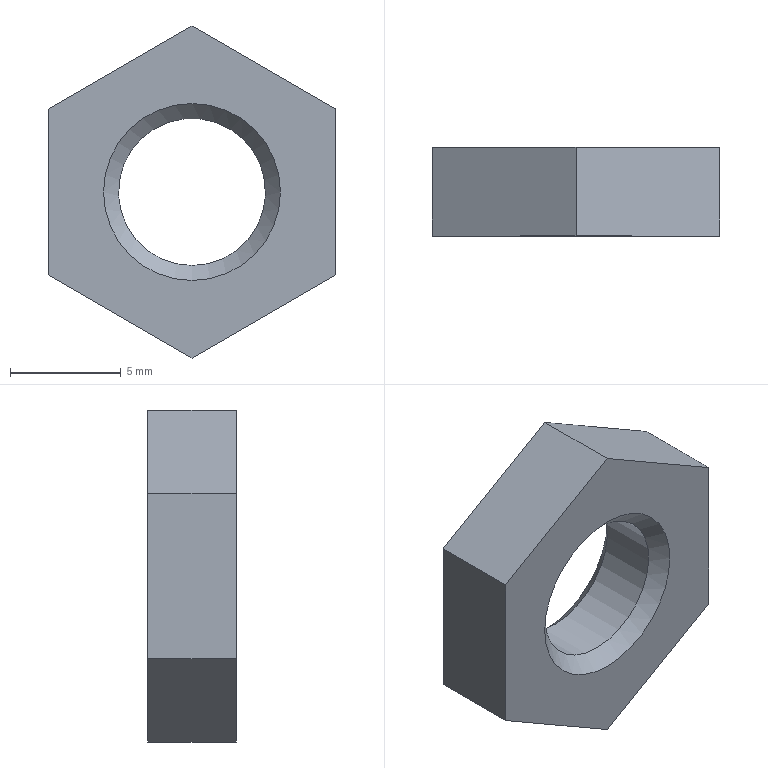Part | STEP file | 1 solid | 11 faces | box 13 x 4 x 15.011 mm | volume 436.424 mm3 | plane 8 | cone 2 | cylinder 1 | commonest cylinder face diameters 6.647 x1
STEP:
#1=CARTESIAN_POINT('',(0.,0.,0.));
#2=DIRECTION('',(0.,0.,1.));
#3=DIRECTION('',(1.,0.,0.));
#4=AXIS2_PLACEMENT_3D('',#1,#2,#3);
#5=CARTESIAN_POINT('',(0.,0.,7.506));
#6=VERTEX_POINT('',#5);
#7=CARTESIAN_POINT('',(6.5,0.,3.753));
#8=VERTEX_POINT('',#7);
#9=CARTESIAN_POINT('',(0.,0.,7.506));
#10=DIRECTION('',(0.866,0.,-0.5));
#11=VECTOR('',#10,1.);
#12=LINE('',#9,#11);
#13=CARTESIAN_POINT('',(0.,0.,7.506));
#14=DIRECTION('',(0.5,0.,0.866));
#15=DIRECTION('',(0.866,0.,-0.5));
#16=AXIS2_PLACEMENT_3D('',#13,#14,#15);
#17=PLANE('',#16);
#18=CARTESIAN_POINT('',(0.,0.));
#19=DIRECTION('',(1.,0.));
#20=VECTOR('',#19,1.);
#21=LINE('',#18,#20);
#22=(GEOMETRIC_REPRESENTATION_CONTEXT(2)PARAMETRIC_REPRESENTATION_CONTEXT()REPRESENTATION_CONTEXT('',''));
#23=DEFINITIONAL_REPRESENTATION('',(#21),#22);
#24=PCURVE('',#17,#23);
#25=CARTESIAN_POINT('',(0.,0.,0.));
#26=DIRECTION('',(0.,1.,0.));
#27=DIRECTION('',(0.,0.,1.));
#28=AXIS2_PLACEMENT_3D('',#25,#26,#27);
#29=PLANE('',#28);
#30=CARTESIAN_POINT('',(7.506,0.));
#31=DIRECTION('',(-0.5,0.866));
#32=VECTOR('',#31,1.);
#33=LINE('',#30,#32);
#34=(GEOMETRIC_REPRESENTATION_CONTEXT(2)PARAMETRIC_REPRESENTATION_CONTEXT()REPRESENTATION_CONTEXT('',''));
#35=DEFINITIONAL_REPRESENTATION('',(#33),#34);
#36=PCURVE('',#29,#35);
#37=SURFACE_CURVE('',#12,(#24,#36),.PCURVE_S1.);
#38=EDGE_CURVE('',#6,#8,#37,.T.);
#39=ORIENTED_EDGE('',*,*,#38,.F.);
#40=CARTESIAN_POINT('',(0.,-4.,7.506));
#41=VERTEX_POINT('',#40);
#42=CARTESIAN_POINT('',(0.,0.,7.506));
#43=DIRECTION('',(0.,-1.,0.));
#44=VECTOR('',#43,1.);
#45=LINE('',#42,#44);
#46=CARTESIAN_POINT('',(0.,0.));
#47=DIRECTION('',(0.,-1.));
#48=VECTOR('',#47,1.);
#49=LINE('',#46,#48);
#50=(GEOMETRIC_REPRESENTATION_CONTEXT(2)PARAMETRIC_REPRESENTATION_CONTEXT()REPRESENTATION_CONTEXT('',''));
#51=DEFINITIONAL_REPRESENTATION('',(#49),#50);
#52=PCURVE('',#17,#51);
#53=CARTESIAN_POINT('',(-6.5,0.,3.753));
#54=DIRECTION('',(-0.5,0.,0.866));
#55=DIRECTION('',(0.866,0.,0.5));
#56=AXIS2_PLACEMENT_3D('',#53,#54,#55);
#57=PLANE('',#56);
#58=CARTESIAN_POINT('',(7.506,0.));
#59=DIRECTION('',(0.,-1.));
#60=VECTOR('',#59,1.);
#61=LINE('',#58,#60);
#62=(GEOMETRIC_REPRESENTATION_CONTEXT(2)PARAMETRIC_REPRESENTATION_CONTEXT()REPRESENTATION_CONTEXT('',''));
#63=DEFINITIONAL_REPRESENTATION('',(#61),#62);
#64=PCURVE('',#57,#63);
#65=SURFACE_CURVE('',#45,(#52,#64),.PCURVE_S1.);
#66=EDGE_CURVE('',#6,#41,#65,.T.);
#67=ORIENTED_EDGE('',*,*,#66,.T.);
#68=CARTESIAN_POINT('',(6.5,-4.,3.753));
#69=VERTEX_POINT('',#68);
#70=CARTESIAN_POINT('',(0.,-4.,7.506));
#71=DIRECTION('',(0.866,0.,-0.5));
#72=VECTOR('',#71,1.);
#73=LINE('',#70,#72);
#74=CARTESIAN_POINT('',(0.,-4.));
#75=DIRECTION('',(1.,0.));
#76=VECTOR('',#75,1.);
#77=LINE('',#74,#76);
#78=(GEOMETRIC_REPRESENTATION_CONTEXT(2)PARAMETRIC_REPRESENTATION_CONTEXT()REPRESENTATION_CONTEXT('',''));
#79=DEFINITIONAL_REPRESENTATION('',(#77),#78);
#80=PCURVE('',#17,#79);
#81=CARTESIAN_POINT('',(0.,-4.,0.));
#82=DIRECTION('',(0.,1.,0.));
#83=DIRECTION('',(0.,0.,1.));
#84=AXIS2_PLACEMENT_3D('',#81,#82,#83);
#85=PLANE('',#84);
#86=CARTESIAN_POINT('',(7.506,0.));
#87=DIRECTION('',(-0.5,0.866));
#88=VECTOR('',#87,1.);
#89=LINE('',#86,#88);
#90=(GEOMETRIC_REPRESENTATION_CONTEXT(2)PARAMETRIC_REPRESENTATION_CONTEXT()REPRESENTATION_CONTEXT('',''));
#91=DEFINITIONAL_REPRESENTATION('',(#89),#90);
#92=PCURVE('',#85,#91);
#93=SURFACE_CURVE('',#73,(#80,#92),.PCURVE_S1.);
#94=EDGE_CURVE('',#41,#69,#93,.T.);
#95=ORIENTED_EDGE('',*,*,#94,.T.);
#96=CARTESIAN_POINT('',(6.5,0.,3.753));
#97=DIRECTION('',(0.,-1.,0.));
#98=VECTOR('',#97,1.);
#99=LINE('',#96,#98);
#100=CARTESIAN_POINT('',(7.506,0.));
#101=DIRECTION('',(0.,-1.));
#102=VECTOR('',#101,1.);
#103=LINE('',#100,#102);
#104=(GEOMETRIC_REPRESENTATION_CONTEXT(2)PARAMETRIC_REPRESENTATION_CONTEXT()REPRESENTATION_CONTEXT('',''));
#105=DEFINITIONAL_REPRESENTATION('',(#103),#104);
#106=PCURVE('',#17,#105);
#107=CARTESIAN_POINT('',(6.5,0.,3.753));
#108=DIRECTION('',(1.,0.,0.));
#109=DIRECTION('',(0.,0.,-1.));
#110=AXIS2_PLACEMENT_3D('',#107,#108,#109);
#111=PLANE('',#110);
#112=CARTESIAN_POINT('',(0.,0.));
#113=DIRECTION('',(0.,-1.));
#114=VECTOR('',#113,1.);
#115=LINE('',#112,#114);
#116=(GEOMETRIC_REPRESENTATION_CONTEXT(2)PARAMETRIC_REPRESENTATION_CONTEXT()REPRESENTATION_CONTEXT('',''));
#117=DEFINITIONAL_REPRESENTATION('',(#115),#116);
#118=PCURVE('',#111,#117);
#119=SURFACE_CURVE('',#99,(#106,#118),.PCURVE_S1.);
#120=EDGE_CURVE('',#8,#69,#119,.T.);
#121=ORIENTED_EDGE('',*,*,#120,.F.);
#122=EDGE_LOOP('',(#39,#67,#95,#121));
#123=FACE_BOUND('',#122,.T.);
#124=ADVANCED_FACE('',(#123),#17,.T.);
#125=CARTESIAN_POINT('',(-6.5,0.,-3.753));
#126=VERTEX_POINT('',#125);
#127=CARTESIAN_POINT('',(-6.5,0.,3.753));
#128=VERTEX_POINT('',#127);
#129=CARTESIAN_POINT('',(-6.5,0.,-3.753));
#130=DIRECTION('',(0.,0.,1.));
#131=VECTOR('',#130,1.);
#132=LINE('',#129,#131);
#133=CARTESIAN_POINT('',(-3.753,-6.5));
#134=DIRECTION('',(1.,0.));
#135=VECTOR('',#134,1.);
#136=LINE('',#133,#135);
#137=(GEOMETRIC_REPRESENTATION_CONTEXT(2)PARAMETRIC_REPRESENTATION_CONTEXT()REPRESENTATION_CONTEXT('',''));
#138=DEFINITIONAL_REPRESENTATION('',(#136),#137);
#139=PCURVE('',#29,#138);
#140=CARTESIAN_POINT('',(-6.5,0.,-3.753));
#141=DIRECTION('',(-1.,0.,0.));
#142=DIRECTION('',(0.,0.,1.));
#143=AXIS2_PLACEMENT_3D('',#140,#141,#142);
#144=PLANE('',#143);
#145=CARTESIAN_POINT('',(0.,0.));
#146=DIRECTION('',(1.,0.));
#147=VECTOR('',#146,1.);
#148=LINE('',#145,#147);
#149=(GEOMETRIC_REPRESENTATION_CONTEXT(2)PARAMETRIC_REPRESENTATION_CONTEXT()REPRESENTATION_CONTEXT('',''));
#150=DEFINITIONAL_REPRESENTATION('',(#148),#149);
#151=PCURVE('',#144,#150);
#152=SURFACE_CURVE('',#132,(#139,#151),.PCURVE_S1.);
#153=EDGE_CURVE('',#126,#128,#152,.T.);
#154=ORIENTED_EDGE('',*,*,#153,.T.);
#155=CARTESIAN_POINT('',(-6.5,0.,3.753));
#156=DIRECTION('',(0.866,0.,0.5));
#157=VECTOR('',#156,1.);
#158=LINE('',#155,#157);
#159=CARTESIAN_POINT('',(3.753,-6.5));
#160=DIRECTION('',(0.5,0.866));
#161=VECTOR('',#160,1.);
#162=LINE('',#159,#161);
#163=(GEOMETRIC_REPRESENTATION_CONTEXT(2)PARAMETRIC_REPRESENTATION_CONTEXT()REPRESENTATION_CONTEXT('',''));
#164=DEFINITIONAL_REPRESENTATION('',(#162),#163);
#165=PCURVE('',#29,#164);
#166=CARTESIAN_POINT('',(0.,0.));
#167=DIRECTION('',(1.,0.));
#168=VECTOR('',#167,1.);
#169=LINE('',#166,#168);
#170=(GEOMETRIC_REPRESENTATION_CONTEXT(2)PARAMETRIC_REPRESENTATION_CONTEXT()REPRESENTATION_CONTEXT('',''));
#171=DEFINITIONAL_REPRESENTATION('',(#169),#170);
#172=PCURVE('',#57,#171);
#173=SURFACE_CURVE('',#158,(#165,#172),.PCURVE_S1.);
#174=EDGE_CURVE('',#128,#6,#173,.T.);
#175=ORIENTED_EDGE('',*,*,#174,.T.);
#176=ORIENTED_EDGE('',*,*,#38,.T.);
#177=CARTESIAN_POINT('',(6.5,0.,-3.753));
#178=VERTEX_POINT('',#177);
#179=CARTESIAN_POINT('',(6.5,0.,3.753));
#180=DIRECTION('',(0.,0.,-1.));
#181=VECTOR('',#180,1.);
#182=LINE('',#179,#181);
#183=CARTESIAN_POINT('',(3.753,6.5));
#184=DIRECTION('',(-1.,0.));
#185=VECTOR('',#184,1.);
#186=LINE('',#183,#185);
#187=(GEOMETRIC_REPRESENTATION_CONTEXT(2)PARAMETRIC_REPRESENTATION_CONTEXT()REPRESENTATION_CONTEXT('',''));
#188=DEFINITIONAL_REPRESENTATION('',(#186),#187);
#189=PCURVE('',#29,#188);
#190=CARTESIAN_POINT('',(0.,0.));
#191=DIRECTION('',(1.,0.));
#192=VECTOR('',#191,1.);
#193=LINE('',#190,#192);
#194=(GEOMETRIC_REPRESENTATION_CONTEXT(2)PARAMETRIC_REPRESENTATION_CONTEXT()REPRESENTATION_CONTEXT('',''));
#195=DEFINITIONAL_REPRESENTATION('',(#193),#194);
#196=PCURVE('',#111,#195);
#197=SURFACE_CURVE('',#182,(#189,#196),.PCURVE_S1.);
#198=EDGE_CURVE('',#8,#178,#197,.T.);
#199=ORIENTED_EDGE('',*,*,#198,.T.);
#200=CARTESIAN_POINT('',(0.,0.,-7.506));
#201=VERTEX_POINT('',#200);
#202=CARTESIAN_POINT('',(6.5,0.,-3.753));
#203=DIRECTION('',(-0.866,0.,-0.5));
#204=VECTOR('',#203,1.);
#205=LINE('',#202,#204);
#206=CARTESIAN_POINT('',(-3.753,6.5));
#207=DIRECTION('',(-0.5,-0.866));
#208=VECTOR('',#207,1.);
#209=LINE('',#206,#208);
#210=(GEOMETRIC_REPRESENTATION_CONTEXT(2)PARAMETRIC_REPRESENTATION_CONTEXT()REPRESENTATION_CONTEXT('',''));
#211=DEFINITIONAL_REPRESENTATION('',(#209),#210);
#212=PCURVE('',#29,#211);
#213=CARTESIAN_POINT('',(6.5,0.,-3.753));
#214=DIRECTION('',(0.5,0.,-0.866));
#215=DIRECTION('',(-0.866,0.,-0.5));
#216=AXIS2_PLACEMENT_3D('',#213,#214,#215);
#217=PLANE('',#216);
#218=CARTESIAN_POINT('',(0.,0.));
#219=DIRECTION('',(1.,0.));
#220=VECTOR('',#219,1.);
#221=LINE('',#218,#220);
#222=(GEOMETRIC_REPRESENTATION_CONTEXT(2)PARAMETRIC_REPRESENTATION_CONTEXT()REPRESENTATION_CONTEXT('',''));
#223=DEFINITIONAL_REPRESENTATION('',(#221),#222);
#224=PCURVE('',#217,#223);
#225=SURFACE_CURVE('',#205,(#212,#224),.PCURVE_S1.);
#226=EDGE_CURVE('',#178,#201,#225,.T.);
#227=ORIENTED_EDGE('',*,*,#226,.T.);
#228=CARTESIAN_POINT('',(0.,0.,-7.506));
#229=DIRECTION('',(-0.866,0.,0.5));
#230=VECTOR('',#229,1.);
#231=LINE('',#228,#230);
#232=CARTESIAN_POINT('',(-7.506,0.));
#233=DIRECTION('',(0.5,-0.866));
#234=VECTOR('',#233,1.);
#235=LINE('',#232,#234);
#236=(GEOMETRIC_REPRESENTATION_CONTEXT(2)PARAMETRIC_REPRESENTATION_CONTEXT()REPRESENTATION_CONTEXT('',''));
#237=DEFINITIONAL_REPRESENTATION('',(#235),#236);
#238=PCURVE('',#29,#237);
#239=CARTESIAN_POINT('',(0.,0.,-7.506));
#240=DIRECTION('',(-0.5,0.,-0.866));
#241=DIRECTION('',(-0.866,0.,0.5));
#242=AXIS2_PLACEMENT_3D('',#239,#240,#241);
#243=PLANE('',#242);
#244=CARTESIAN_POINT('',(0.,0.));
#245=DIRECTION('',(1.,0.));
#246=VECTOR('',#245,1.);
#247=LINE('',#244,#246);
#248=(GEOMETRIC_REPRESENTATION_CONTEXT(2)PARAMETRIC_REPRESENTATION_CONTEXT()REPRESENTATION_CONTEXT('',''));
#249=DEFINITIONAL_REPRESENTATION('',(#247),#248);
#250=PCURVE('',#243,#249);
#251=SURFACE_CURVE('',#231,(#238,#250),.PCURVE_S1.);
#252=EDGE_CURVE('',#201,#126,#251,.T.);
#253=ORIENTED_EDGE('',*,*,#252,.T.);
#254=EDGE_LOOP('',(#154,#175,#176,#199,#227,#253));
#255=FACE_BOUND('',#254,.T.);
#256=CARTESIAN_POINT('',(0.,0.,-4.));
#257=VERTEX_POINT('',#256);
#258=CARTESIAN_POINT('',(0.,0.,0.));
#259=DIRECTION('',(0.,1.,0.));
#260=DIRECTION('',(1.,0.,0.));
#261=AXIS2_PLACEMENT_3D('',#258,#259,#260);
#262=CIRCLE('',#261,4.);
#263=CARTESIAN_POINT('',(0.,0.));
#264=DIRECTION('',(0.,1.));
#265=AXIS2_PLACEMENT_2D('',#263,#264);
#266=CIRCLE('',#265,4.);
#267=(GEOMETRIC_REPRESENTATION_CONTEXT(2)PARAMETRIC_REPRESENTATION_CONTEXT()REPRESENTATION_CONTEXT('',''));
#268=DEFINITIONAL_REPRESENTATION('',(#266),#267);
#269=PCURVE('',#29,#268);
#270=CARTESIAN_POINT('',(0.,1.,0.));
#271=DIRECTION('',(0.,1.,0.));
#272=DIRECTION('',(0.,0.,1.));
#273=AXIS2_PLACEMENT_3D('',#270,#271,#272);
#274=CONICAL_SURFACE('',#273,5.,0.7854);
#275=CARTESIAN_POINT('',(1.571,-1.));
#276=DIRECTION('',(1.,0.));
#277=VECTOR('',#276,1.);
#278=LINE('',#275,#277);
#279=(GEOMETRIC_REPRESENTATION_CONTEXT(2)PARAMETRIC_REPRESENTATION_CONTEXT()REPRESENTATION_CONTEXT('',''));
#280=DEFINITIONAL_REPRESENTATION('',(#278),#279);
#281=PCURVE('',#274,#280);
#282=SURFACE_CURVE('',#262,(#269,#281),.PCURVE_S1.);
#283=EDGE_CURVE('',#257,#257,#282,.T.);
#284=ORIENTED_EDGE('',*,*,#283,.F.);
#285=EDGE_LOOP('',(#284));
#286=FACE_BOUND('',#285,.T.);
#287=ADVANCED_FACE('',(#255,#286),#29,.T.);
#288=ORIENTED_EDGE('',*,*,#174,.F.);
#289=CARTESIAN_POINT('',(-6.5,-4.,3.753));
#290=VERTEX_POINT('',#289);
#291=CARTESIAN_POINT('',(-6.5,0.,3.753));
#292=DIRECTION('',(0.,-1.,0.));
#293=VECTOR('',#292,1.);
#294=LINE('',#291,#293);
#295=CARTESIAN_POINT('',(0.,0.));
#296=DIRECTION('',(0.,-1.));
#297=VECTOR('',#296,1.);
#298=LINE('',#295,#297);
#299=(GEOMETRIC_REPRESENTATION_CONTEXT(2)PARAMETRIC_REPRESENTATION_CONTEXT()REPRESENTATION_CONTEXT('',''));
#300=DEFINITIONAL_REPRESENTATION('',(#298),#299);
#301=PCURVE('',#57,#300);
#302=CARTESIAN_POINT('',(7.506,0.));
#303=DIRECTION('',(0.,-1.));
#304=VECTOR('',#303,1.);
#305=LINE('',#302,#304);
#306=(GEOMETRIC_REPRESENTATION_CONTEXT(2)PARAMETRIC_REPRESENTATION_CONTEXT()REPRESENTATION_CONTEXT('',''));
#307=DEFINITIONAL_REPRESENTATION('',(#305),#306);
#308=PCURVE('',#144,#307);
#309=SURFACE_CURVE('',#294,(#301,#308),.PCURVE_S1.);
#310=EDGE_CURVE('',#128,#290,#309,.T.);
#311=ORIENTED_EDGE('',*,*,#310,.T.);
#312=CARTESIAN_POINT('',(-6.5,-4.,3.753));
#313=DIRECTION('',(0.866,0.,0.5));
#314=VECTOR('',#313,1.);
#315=LINE('',#312,#314);
#316=CARTESIAN_POINT('',(0.,-4.));
#317=DIRECTION('',(1.,0.));
#318=VECTOR('',#317,1.);
#319=LINE('',#316,#318);
#320=(GEOMETRIC_REPRESENTATION_CONTEXT(2)PARAMETRIC_REPRESENTATION_CONTEXT()REPRESENTATION_CONTEXT('',''));
#321=DEFINITIONAL_REPRESENTATION('',(#319),#320);
#322=PCURVE('',#57,#321);
#323=CARTESIAN_POINT('',(3.753,-6.5));
#324=DIRECTION('',(0.5,0.866));
#325=VECTOR('',#324,1.);
#326=LINE('',#323,#325);
#327=(GEOMETRIC_REPRESENTATION_CONTEXT(2)PARAMETRIC_REPRESENTATION_CONTEXT()REPRESENTATION_CONTEXT('',''));
#328=DEFINITIONAL_REPRESENTATION('',(#326),#327);
#329=PCURVE('',#85,#328);
#330=SURFACE_CURVE('',#315,(#322,#329),.PCURVE_S1.);
#331=EDGE_CURVE('',#290,#41,#330,.T.);
#332=ORIENTED_EDGE('',*,*,#331,.T.);
#333=ORIENTED_EDGE('',*,*,#66,.F.);
#334=EDGE_LOOP('',(#288,#311,#332,#333));
#335=FACE_BOUND('',#334,.T.);
#336=ADVANCED_FACE('',(#335),#57,.T.);
#337=CARTESIAN_POINT('',(0.,-4.,-7.506));
#338=VERTEX_POINT('',#337);
#339=CARTESIAN_POINT('',(-6.5,-4.,-3.753));
#340=VERTEX_POINT('',#339);
#341=CARTESIAN_POINT('',(0.,-4.,-7.506));
#342=DIRECTION('',(-0.866,0.,0.5));
#343=VECTOR('',#342,1.);
#344=LINE('',#341,#343);
#345=CARTESIAN_POINT('',(-7.506,0.));
#346=DIRECTION('',(0.5,-0.866));
#347=VECTOR('',#346,1.);
#348=LINE('',#345,#347);
#349=(GEOMETRIC_REPRESENTATION_CONTEXT(2)PARAMETRIC_REPRESENTATION_CONTEXT()REPRESENTATION_CONTEXT('',''));
#350=DEFINITIONAL_REPRESENTATION('',(#348),#349);
#351=PCURVE('',#85,#350);
#352=CARTESIAN_POINT('',(0.,-4.));
#353=DIRECTION('',(1.,0.));
#354=VECTOR('',#353,1.);
#355=LINE('',#352,#354);
#356=(GEOMETRIC_REPRESENTATION_CONTEXT(2)PARAMETRIC_REPRESENTATION_CONTEXT()REPRESENTATION_CONTEXT('',''));
#357=DEFINITIONAL_REPRESENTATION('',(#355),#356);
#358=PCURVE('',#243,#357);
#359=SURFACE_CURVE('',#344,(#351,#358),.PCURVE_S1.);
#360=EDGE_CURVE('',#338,#340,#359,.T.);
#361=ORIENTED_EDGE('',*,*,#360,.F.);
#362=CARTESIAN_POINT('',(6.5,-4.,-3.753));
#363=VERTEX_POINT('',#362);
#364=CARTESIAN_POINT('',(6.5,-4.,-3.753));
#365=DIRECTION('',(-0.866,0.,-0.5));
#366=VECTOR('',#365,1.);
#367=LINE('',#364,#366);
#368=CARTESIAN_POINT('',(-3.753,6.5));
#369=DIRECTION('',(-0.5,-0.866));
#370=VECTOR('',#369,1.);
#371=LINE('',#368,#370);
#372=(GEOMETRIC_REPRESENTATION_CONTEXT(2)PARAMETRIC_REPRESENTATION_CONTEXT()REPRESENTATION_CONTEXT('',''));
#373=DEFINITIONAL_REPRESENTATION('',(#371),#372);
#374=PCURVE('',#85,#373);
#375=CARTESIAN_POINT('',(0.,-4.));
#376=DIRECTION('',(1.,0.));
#377=VECTOR('',#376,1.);
#378=LINE('',#375,#377);
#379=(GEOMETRIC_REPRESENTATION_CONTEXT(2)PARAMETRIC_REPRESENTATION_CONTEXT()REPRESENTATION_CONTEXT('',''));
#380=DEFINITIONAL_REPRESENTATION('',(#378),#379);
#381=PCURVE('',#217,#380);
#382=SURFACE_CURVE('',#367,(#374,#381),.PCURVE_S1.);
#383=EDGE_CURVE('',#363,#338,#382,.T.);
#384=ORIENTED_EDGE('',*,*,#383,.F.);
#385=CARTESIAN_POINT('',(6.5,-4.,3.753));
#386=DIRECTION('',(0.,0.,-1.));
#387=VECTOR('',#386,1.);
#388=LINE('',#385,#387);
#389=CARTESIAN_POINT('',(3.753,6.5));
#390=DIRECTION('',(-1.,0.));
#391=VECTOR('',#390,1.);
#392=LINE('',#389,#391);
#393=(GEOMETRIC_REPRESENTATION_CONTEXT(2)PARAMETRIC_REPRESENTATION_CONTEXT()REPRESENTATION_CONTEXT('',''));
#394=DEFINITIONAL_REPRESENTATION('',(#392),#393);
#395=PCURVE('',#85,#394);
#396=CARTESIAN_POINT('',(0.,-4.));
#397=DIRECTION('',(1.,0.));
#398=VECTOR('',#397,1.);
#399=LINE('',#396,#398);
#400=(GEOMETRIC_REPRESENTATION_CONTEXT(2)PARAMETRIC_REPRESENTATION_CONTEXT()REPRESENTATION_CONTEXT('',''));
#401=DEFINITIONAL_REPRESENTATION('',(#399),#400);
#402=PCURVE('',#111,#401);
#403=SURFACE_CURVE('',#388,(#395,#402),.PCURVE_S1.);
#404=EDGE_CURVE('',#69,#363,#403,.T.);
#405=ORIENTED_EDGE('',*,*,#404,.F.);
#406=ORIENTED_EDGE('',*,*,#94,.F.);
#407=ORIENTED_EDGE('',*,*,#331,.F.);
#408=CARTESIAN_POINT('',(-6.5,-4.,-3.753));
#409=DIRECTION('',(0.,0.,1.));
#410=VECTOR('',#409,1.);
#411=LINE('',#408,#410);
#412=CARTESIAN_POINT('',(-3.753,-6.5));
#413=DIRECTION('',(1.,0.));
#414=VECTOR('',#413,1.);
#415=LINE('',#412,#414);
#416=(GEOMETRIC_REPRESENTATION_CONTEXT(2)PARAMETRIC_REPRESENTATION_CONTEXT()REPRESENTATION_CONTEXT('',''));
#417=DEFINITIONAL_REPRESENTATION('',(#415),#416);
#418=PCURVE('',#85,#417);
#419=CARTESIAN_POINT('',(0.,-4.));
#420=DIRECTION('',(1.,0.));
#421=VECTOR('',#420,1.);
#422=LINE('',#419,#421);
#423=(GEOMETRIC_REPRESENTATION_CONTEXT(2)PARAMETRIC_REPRESENTATION_CONTEXT()REPRESENTATION_CONTEXT('',''));
#424=DEFINITIONAL_REPRESENTATION('',(#422),#423);
#425=PCURVE('',#144,#424);
#426=SURFACE_CURVE('',#411,(#418,#425),.PCURVE_S1.);
#427=EDGE_CURVE('',#340,#290,#426,.T.);
#428=ORIENTED_EDGE('',*,*,#427,.F.);
#429=EDGE_LOOP('',(#361,#384,#405,#406,#407,#428));
#430=FACE_BOUND('',#429,.T.);
#431=CARTESIAN_POINT('',(0.,-4.,-4.));
#432=VERTEX_POINT('',#431);
#433=CARTESIAN_POINT('',(0.,-4.,0.));
#434=DIRECTION('',(0.,-1.,0.));
#435=DIRECTION('',(0.,0.,1.));
#436=AXIS2_PLACEMENT_3D('',#433,#434,#435);
#437=CIRCLE('',#436,4.);
#438=CARTESIAN_POINT('',(4.,0.));
#439=CARTESIAN_POINT('',(4.,-6.928));
#440=CARTESIAN_POINT('',(-2.,-3.464));
#441=CARTESIAN_POINT('',(-8.,0.));
#442=CARTESIAN_POINT('',(-2.,3.464));
#443=CARTESIAN_POINT('',(4.,6.928));
#444=CARTESIAN_POINT('',(4.,0.));
#445=(BOUNDED_CURVE()B_SPLINE_CURVE(2,(#438,#439,#440,#441,#442,#443,#444),.UNSPECIFIED.,.T.,.F.)B_SPLINE_CURVE_WITH_KNOTS((1,2,2,2,2,1),(-2.094,0.,2.094,4.189,6.283,8.378),.UNSPECIFIED.)CURVE()GEOMETRIC_REPRESENTATION_ITEM()RATIONAL_B_SPLINE_CURVE((1.,0.5,1.,0.5,1.,0.5,1.))REPRESENTATION_ITEM(''));
#446=(GEOMETRIC_REPRESENTATION_CONTEXT(2)PARAMETRIC_REPRESENTATION_CONTEXT()REPRESENTATION_CONTEXT('',''));
#447=DEFINITIONAL_REPRESENTATION('',(#445),#446);
#448=PCURVE('',#85,#447);
#449=CARTESIAN_POINT('',(0.,-5.,0.));
#450=DIRECTION('',(0.,-1.,0.));
#451=DIRECTION('',(0.,0.,-1.));
#452=AXIS2_PLACEMENT_3D('',#449,#450,#451);
#453=CONICAL_SURFACE('',#452,5.,0.7854);
#454=CARTESIAN_POINT('',(-3.142,-1.));
#455=DIRECTION('',(1.,0.));
#456=VECTOR('',#455,1.);
#457=LINE('',#454,#456);
#458=(GEOMETRIC_REPRESENTATION_CONTEXT(2)PARAMETRIC_REPRESENTATION_CONTEXT()REPRESENTATION_CONTEXT('',''));
#459=DEFINITIONAL_REPRESENTATION('',(#457),#458);
#460=PCURVE('',#453,#459);
#461=SURFACE_CURVE('',#437,(#448,#460),.PCURVE_S1.);
#462=EDGE_CURVE('',#432,#432,#461,.T.);
#463=ORIENTED_EDGE('',*,*,#462,.F.);
#464=EDGE_LOOP('',(#463));
#465=FACE_BOUND('',#464,.T.);
#466=ADVANCED_FACE('',(#430,#465),#85,.F.);
#467=ORIENTED_EDGE('',*,*,#198,.F.);
#468=ORIENTED_EDGE('',*,*,#120,.T.);
#469=ORIENTED_EDGE('',*,*,#404,.T.);
#470=CARTESIAN_POINT('',(6.5,0.,-3.753));
#471=DIRECTION('',(0.,-1.,0.));
#472=VECTOR('',#471,1.);
#473=LINE('',#470,#472);
#474=CARTESIAN_POINT('',(7.506,0.));
#475=DIRECTION('',(0.,-1.));
#476=VECTOR('',#475,1.);
#477=LINE('',#474,#476);
#478=(GEOMETRIC_REPRESENTATION_CONTEXT(2)PARAMETRIC_REPRESENTATION_CONTEXT()REPRESENTATION_CONTEXT('',''));
#479=DEFINITIONAL_REPRESENTATION('',(#477),#478);
#480=PCURVE('',#111,#479);
#481=CARTESIAN_POINT('',(0.,0.));
#482=DIRECTION('',(0.,-1.));
#483=VECTOR('',#482,1.);
#484=LINE('',#481,#483);
#485=(GEOMETRIC_REPRESENTATION_CONTEXT(2)PARAMETRIC_REPRESENTATION_CONTEXT()REPRESENTATION_CONTEXT('',''));
#486=DEFINITIONAL_REPRESENTATION('',(#484),#485);
#487=PCURVE('',#217,#486);
#488=SURFACE_CURVE('',#473,(#480,#487),.PCURVE_S1.);
#489=EDGE_CURVE('',#178,#363,#488,.T.);
#490=ORIENTED_EDGE('',*,*,#489,.F.);
#491=EDGE_LOOP('',(#467,#468,#469,#490));
#492=FACE_BOUND('',#491,.T.);
#493=ADVANCED_FACE('',(#492),#111,.T.);
#494=ORIENTED_EDGE('',*,*,#153,.F.);
#495=CARTESIAN_POINT('',(-6.5,0.,-3.753));
#496=DIRECTION('',(0.,-1.,0.));
#497=VECTOR('',#496,1.);
#498=LINE('',#495,#497);
#499=CARTESIAN_POINT('',(0.,0.));
#500=DIRECTION('',(0.,-1.));
#501=VECTOR('',#500,1.);
#502=LINE('',#499,#501);
#503=(GEOMETRIC_REPRESENTATION_CONTEXT(2)PARAMETRIC_REPRESENTATION_CONTEXT()REPRESENTATION_CONTEXT('',''));
#504=DEFINITIONAL_REPRESENTATION('',(#502),#503);
#505=PCURVE('',#144,#504);
#506=CARTESIAN_POINT('',(7.506,0.));
#507=DIRECTION('',(0.,-1.));
#508=VECTOR('',#507,1.);
#509=LINE('',#506,#508);
#510=(GEOMETRIC_REPRESENTATION_CONTEXT(2)PARAMETRIC_REPRESENTATION_CONTEXT()REPRESENTATION_CONTEXT('',''));
#511=DEFINITIONAL_REPRESENTATION('',(#509),#510);
#512=PCURVE('',#243,#511);
#513=SURFACE_CURVE('',#498,(#505,#512),.PCURVE_S1.);
#514=EDGE_CURVE('',#126,#340,#513,.T.);
#515=ORIENTED_EDGE('',*,*,#514,.T.);
#516=ORIENTED_EDGE('',*,*,#427,.T.);
#517=ORIENTED_EDGE('',*,*,#310,.F.);
#518=EDGE_LOOP('',(#494,#515,#516,#517));
#519=FACE_BOUND('',#518,.T.);
#520=ADVANCED_FACE('',(#519),#144,.T.);
#521=ORIENTED_EDGE('',*,*,#226,.F.);
#522=ORIENTED_EDGE('',*,*,#489,.T.);
#523=ORIENTED_EDGE('',*,*,#383,.T.);
#524=CARTESIAN_POINT('',(0.000000001,0.,-7.506));
#525=DIRECTION('',(0.,-1.,0.));
#526=VECTOR('',#525,1.);
#527=LINE('',#524,#526);
#528=CARTESIAN_POINT('',(7.506,0.));
#529=DIRECTION('',(0.,-1.));
#530=VECTOR('',#529,1.);
#531=LINE('',#528,#530);
#532=(GEOMETRIC_REPRESENTATION_CONTEXT(2)PARAMETRIC_REPRESENTATION_CONTEXT()REPRESENTATION_CONTEXT('',''));
#533=DEFINITIONAL_REPRESENTATION('',(#531),#532);
#534=PCURVE('',#217,#533);
#535=CARTESIAN_POINT('',(0.,0.));
#536=DIRECTION('',(0.,-1.));
#537=VECTOR('',#536,1.);
#538=LINE('',#535,#537);
#539=(GEOMETRIC_REPRESENTATION_CONTEXT(2)PARAMETRIC_REPRESENTATION_CONTEXT()REPRESENTATION_CONTEXT('',''));
#540=DEFINITIONAL_REPRESENTATION('',(#538),#539);
#541=PCURVE('',#243,#540);
#542=SURFACE_CURVE('',#527,(#534,#541),.PCURVE_S1.);
#543=EDGE_CURVE('',#201,#338,#542,.T.);
#544=ORIENTED_EDGE('',*,*,#543,.F.);
#545=EDGE_LOOP('',(#521,#522,#523,#544));
#546=FACE_BOUND('',#545,.T.);
#547=ADVANCED_FACE('',(#546),#217,.T.);
#548=ORIENTED_EDGE('',*,*,#252,.F.);
#549=ORIENTED_EDGE('',*,*,#543,.T.);
#550=ORIENTED_EDGE('',*,*,#360,.T.);
#551=ORIENTED_EDGE('',*,*,#514,.F.);
#552=EDGE_LOOP('',(#548,#549,#550,#551));
#553=FACE_BOUND('',#552,.T.);
#554=ADVANCED_FACE('',(#553),#243,.T.);
#555=CARTESIAN_POINT('',(0.,-0.6765,-3.324));
#556=VERTEX_POINT('',#555);
#557=CARTESIAN_POINT('',(0.,-0.6765,0.));
#558=DIRECTION('',(0.,1.,0.));
#559=DIRECTION('',(1.,0.,0.));
#560=AXIS2_PLACEMENT_3D('',#557,#558,#559);
#561=CIRCLE('',#560,3.324);
#562=CARTESIAN_POINT('',(1.571,-1.677));
#563=DIRECTION('',(1.,0.));
#564=VECTOR('',#563,1.);
#565=LINE('',#562,#564);
#566=(GEOMETRIC_REPRESENTATION_CONTEXT(2)PARAMETRIC_REPRESENTATION_CONTEXT()REPRESENTATION_CONTEXT('',''));
#567=DEFINITIONAL_REPRESENTATION('',(#565),#566);
#568=PCURVE('',#274,#567);
#569=CARTESIAN_POINT('',(0.,-2.,0.));
#570=DIRECTION('',(0.,1.,0.));
#571=DIRECTION('',(0.,0.,1.));
#572=AXIS2_PLACEMENT_3D('',#569,#570,#571);
#573=CYLINDRICAL_SURFACE('',#572,3.324);
#574=CARTESIAN_POINT('',(1.571,1.323));
#575=DIRECTION('',(1.,0.));
#576=VECTOR('',#575,1.);
#577=LINE('',#574,#576);
#578=(GEOMETRIC_REPRESENTATION_CONTEXT(2)PARAMETRIC_REPRESENTATION_CONTEXT()REPRESENTATION_CONTEXT('',''));
#579=DEFINITIONAL_REPRESENTATION('',(#577),#578);
#580=PCURVE('',#573,#579);
#581=SURFACE_CURVE('',#561,(#568,#580),.PCURVE_S1.);
#582=EDGE_CURVE('',#556,#556,#581,.T.);
#583=ORIENTED_EDGE('',*,*,#582,.T.);
#584=CARTESIAN_POINT('',(0.,-0.6765,-3.324));
#585=CARTESIAN_POINT('',(0.,-0.000000001,-4.));
#586=B_SPLINE_CURVE_WITH_KNOTS('',1,(#584,#585),.UNSPECIFIED.,.F.,.F.,(2,2),(-2.371,-1.414),.PIECEWISE_BEZIER_KNOTS.);
#587=CARTESIAN_POINT('',(9.425,0.));
#588=DIRECTION('',(0.,1.));
#589=VECTOR('',#588,1.);
#590=LINE('',#587,#589);
#591=(GEOMETRIC_REPRESENTATION_CONTEXT(2)PARAMETRIC_REPRESENTATION_CONTEXT()REPRESENTATION_CONTEXT('',''));
#592=DEFINITIONAL_REPRESENTATION('',(#590),#591);
#593=PCURVE('',#274,#592);
#594=CARTESIAN_POINT('',(3.142,0.));
#595=DIRECTION('',(0.,1.));
#596=VECTOR('',#595,1.);
#597=LINE('',#594,#596);
#598=(GEOMETRIC_REPRESENTATION_CONTEXT(2)PARAMETRIC_REPRESENTATION_CONTEXT()REPRESENTATION_CONTEXT('',''));
#599=DEFINITIONAL_REPRESENTATION('',(#597),#598);
#600=PCURVE('',#274,#599);
#601=SEAM_CURVE('',#586,(#593,#600),.PCURVE_S1.);
#602=EDGE_CURVE('',#556,#257,#601,.T.);
#603=ORIENTED_EDGE('',*,*,#602,.T.);
#604=ORIENTED_EDGE('',*,*,#283,.F.);
#605=ORIENTED_EDGE('',*,*,#602,.F.);
#606=EDGE_LOOP('',(#583,#603,#604,#605));
#607=FACE_BOUND('',#606,.F.);
#608=ADVANCED_FACE('',(#607),#274,.F.);
#609=ORIENTED_EDGE('',*,*,#462,.F.);
#610=CARTESIAN_POINT('',(0.,-3.324,-3.324));
#611=VERTEX_POINT('',#610);
#612=CARTESIAN_POINT('',(0.,-3.323,-3.324));
#613=CARTESIAN_POINT('',(0.,-4.,-4.));
#614=B_SPLINE_CURVE_WITH_KNOTS('',1,(#612,#613),.UNSPECIFIED.,.F.,.F.,(2,2),(-2.371,-1.414),.PIECEWISE_BEZIER_KNOTS.);
#615=CARTESIAN_POINT('',(0.,0.));
#616=DIRECTION('',(0.,1.));
#617=VECTOR('',#616,1.);
#618=LINE('',#615,#617);
#619=(GEOMETRIC_REPRESENTATION_CONTEXT(2)PARAMETRIC_REPRESENTATION_CONTEXT()REPRESENTATION_CONTEXT('',''));
#620=DEFINITIONAL_REPRESENTATION('',(#618),#619);
#621=PCURVE('',#453,#620);
#622=CARTESIAN_POINT('',(6.283,0.));
#623=DIRECTION('',(0.,1.));
#624=VECTOR('',#623,1.);
#625=LINE('',#622,#624);
#626=(GEOMETRIC_REPRESENTATION_CONTEXT(2)PARAMETRIC_REPRESENTATION_CONTEXT()REPRESENTATION_CONTEXT('',''));
#627=DEFINITIONAL_REPRESENTATION('',(#625),#626);
#628=PCURVE('',#453,#627);
#629=SEAM_CURVE('',#614,(#621,#628),.PCURVE_S1.);
#630=EDGE_CURVE('',#611,#432,#629,.T.);
#631=ORIENTED_EDGE('',*,*,#630,.F.);
#632=CARTESIAN_POINT('',(0.,-3.324,0.));
#633=DIRECTION('',(0.,-1.,0.));
#634=DIRECTION('',(1.,0.,0.));
#635=AXIS2_PLACEMENT_3D('',#632,#633,#634);
#636=CIRCLE('',#635,3.324);
#637=CARTESIAN_POINT('',(-4.712,-1.677));
#638=DIRECTION('',(1.,0.));
#639=VECTOR('',#638,1.);
#640=LINE('',#637,#639);
#641=(GEOMETRIC_REPRESENTATION_CONTEXT(2)PARAMETRIC_REPRESENTATION_CONTEXT()REPRESENTATION_CONTEXT('',''));
#642=DEFINITIONAL_REPRESENTATION('',(#640),#641);
#643=PCURVE('',#453,#642);
#644=CARTESIAN_POINT('',(14.137,-1.323));
#645=DIRECTION('',(-1.,0.));
#646=VECTOR('',#645,1.);
#647=LINE('',#644,#646);
#648=(GEOMETRIC_REPRESENTATION_CONTEXT(2)PARAMETRIC_REPRESENTATION_CONTEXT()REPRESENTATION_CONTEXT('',''));
#649=DEFINITIONAL_REPRESENTATION('',(#647),#648);
#650=PCURVE('',#573,#649);
#651=SURFACE_CURVE('',#636,(#643,#650),.PCURVE_S1.);
#652=EDGE_CURVE('',#611,#611,#651,.T.);
#653=ORIENTED_EDGE('',*,*,#652,.T.);
#654=ORIENTED_EDGE('',*,*,#630,.T.);
#655=EDGE_LOOP('',(#609,#631,#653,#654));
#656=FACE_BOUND('',#655,.F.);
#657=ADVANCED_FACE('',(#656),#453,.F.);
#658=ORIENTED_EDGE('',*,*,#652,.F.);
#659=CARTESIAN_POINT('',(0.,-3.324,-3.324));
#660=CARTESIAN_POINT('',(0.,-0.6765,-3.324));
#661=B_SPLINE_CURVE_WITH_KNOTS('',1,(#659,#660),.UNSPECIFIED.,.F.,.F.,(2,2),(-1.323,1.323),.PIECEWISE_BEZIER_KNOTS.);
#662=CARTESIAN_POINT('',(9.425,0.));
#663=DIRECTION('',(0.,1.));
#664=VECTOR('',#663,1.);
#665=LINE('',#662,#664);
#666=(GEOMETRIC_REPRESENTATION_CONTEXT(2)PARAMETRIC_REPRESENTATION_CONTEXT()REPRESENTATION_CONTEXT('',''));
#667=DEFINITIONAL_REPRESENTATION('',(#665),#666);
#668=PCURVE('',#573,#667);
#669=CARTESIAN_POINT('',(3.142,0.));
#670=DIRECTION('',(0.,1.));
#671=VECTOR('',#670,1.);
#672=LINE('',#669,#671);
#673=(GEOMETRIC_REPRESENTATION_CONTEXT(2)PARAMETRIC_REPRESENTATION_CONTEXT()REPRESENTATION_CONTEXT('',''));
#674=DEFINITIONAL_REPRESENTATION('',(#672),#673);
#675=PCURVE('',#573,#674);
#676=SEAM_CURVE('',#661,(#668,#675),.PCURVE_S1.);
#677=EDGE_CURVE('',#611,#556,#676,.T.);
#678=ORIENTED_EDGE('',*,*,#677,.T.);
#679=ORIENTED_EDGE('',*,*,#582,.F.);
#680=ORIENTED_EDGE('',*,*,#677,.F.);
#681=EDGE_LOOP('',(#658,#678,#679,#680));
#682=FACE_BOUND('',#681,.F.);
#683=ADVANCED_FACE('',(#682),#573,.F.);
#684=CLOSED_SHELL('',(#124,#287,#336,#466,#493,#520,#547,#554,#608,#657,#683));
#685=MANIFOLD_SOLID_BREP('',#684);
#686=(LENGTH_UNIT()NAMED_UNIT(*)SI_UNIT(.MILLI.,.METRE.));
#687=UNCERTAINTY_MEASURE_WITH_UNIT(LENGTH_MEASURE(0.000002),#686,'','');
#688=(NAMED_UNIT(*)PLANE_ANGLE_UNIT()SI_UNIT($,.RADIAN.));
#689=(NAMED_UNIT(*)SI_UNIT($,.STERADIAN.)SOLID_ANGLE_UNIT());
#690=(GEOMETRIC_REPRESENTATION_CONTEXT(3)GLOBAL_UNCERTAINTY_ASSIGNED_CONTEXT((#687))GLOBAL_UNIT_ASSIGNED_CONTEXT((#686,#688,#689))REPRESENTATION_CONTEXT('',''));
#691=ADVANCED_BREP_SHAPE_REPRESENTATION('',(#4,#685),#690);